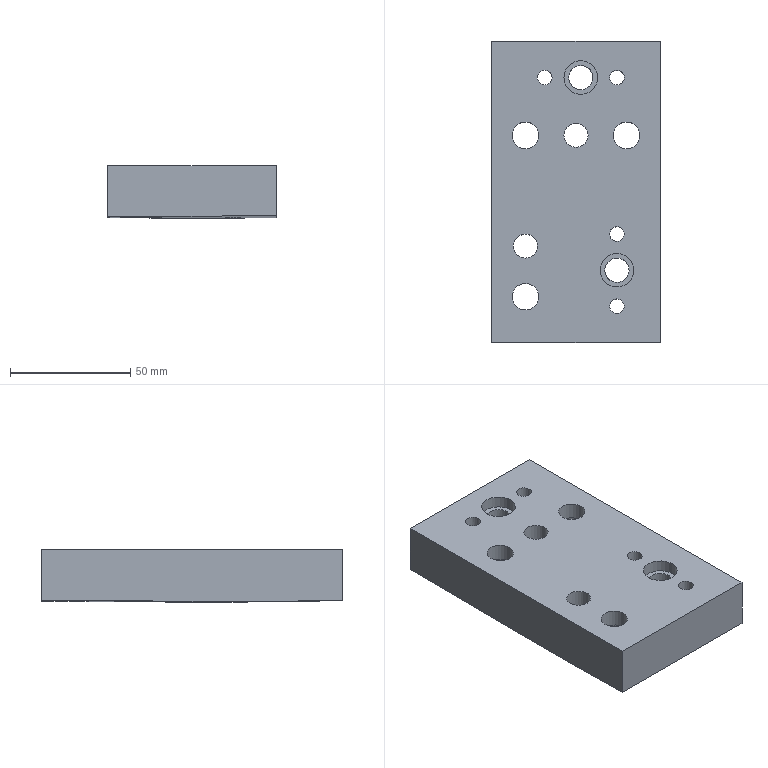Part | STEP file | 416_id1198_x_t | 1 solid | 31 faces | box 70 x 125 x 21.726 mm | volume 164962 mm3 | cylinder 18 | plane 12 | spline 1 | commonest cylinder face diameters 6.1 x4 11 x3 17 x3 10 x2 10.1 x2 12 x2